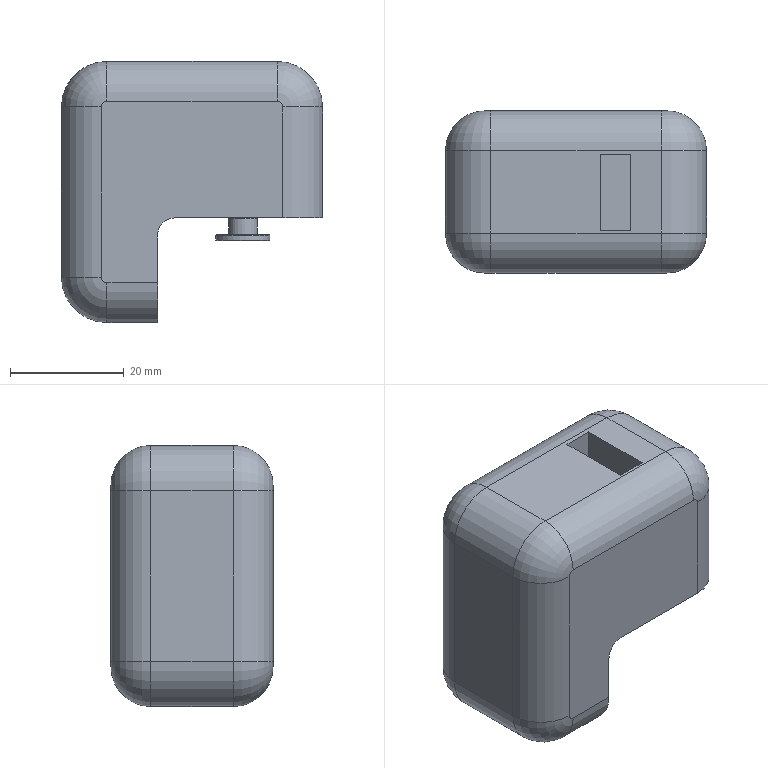Part | STEP file | Product-2 | 1 solid | 64 faces | box 45.9 x 28.5 x 45.9 mm | volume 40224 mm3 | cylinder 24 | plane 20 | spline 10 | torus 10 | commonest cylinder face diameters 14 x8 2 x4 16 x3 0.6 x2 4.85 x2 5 x2